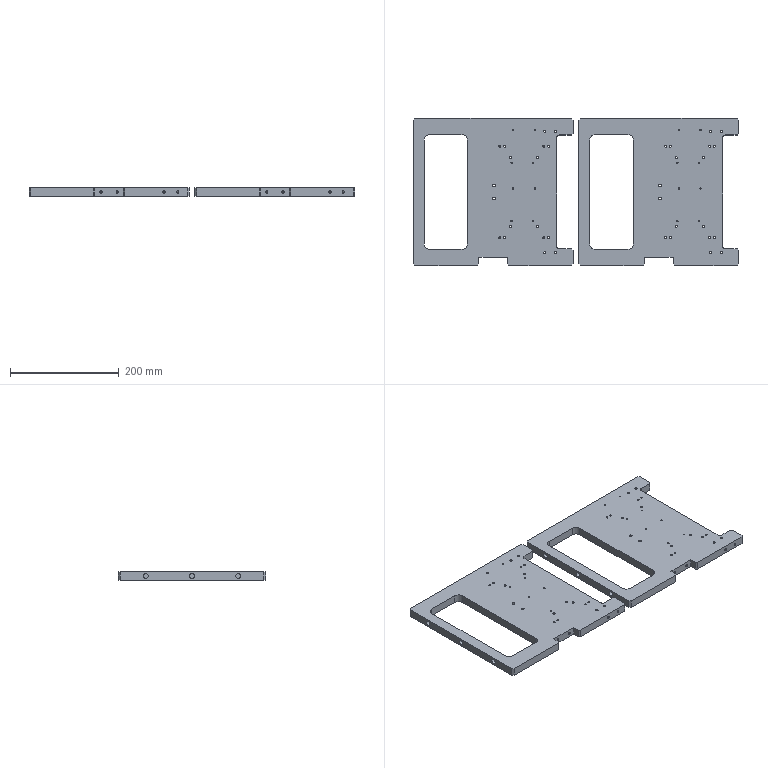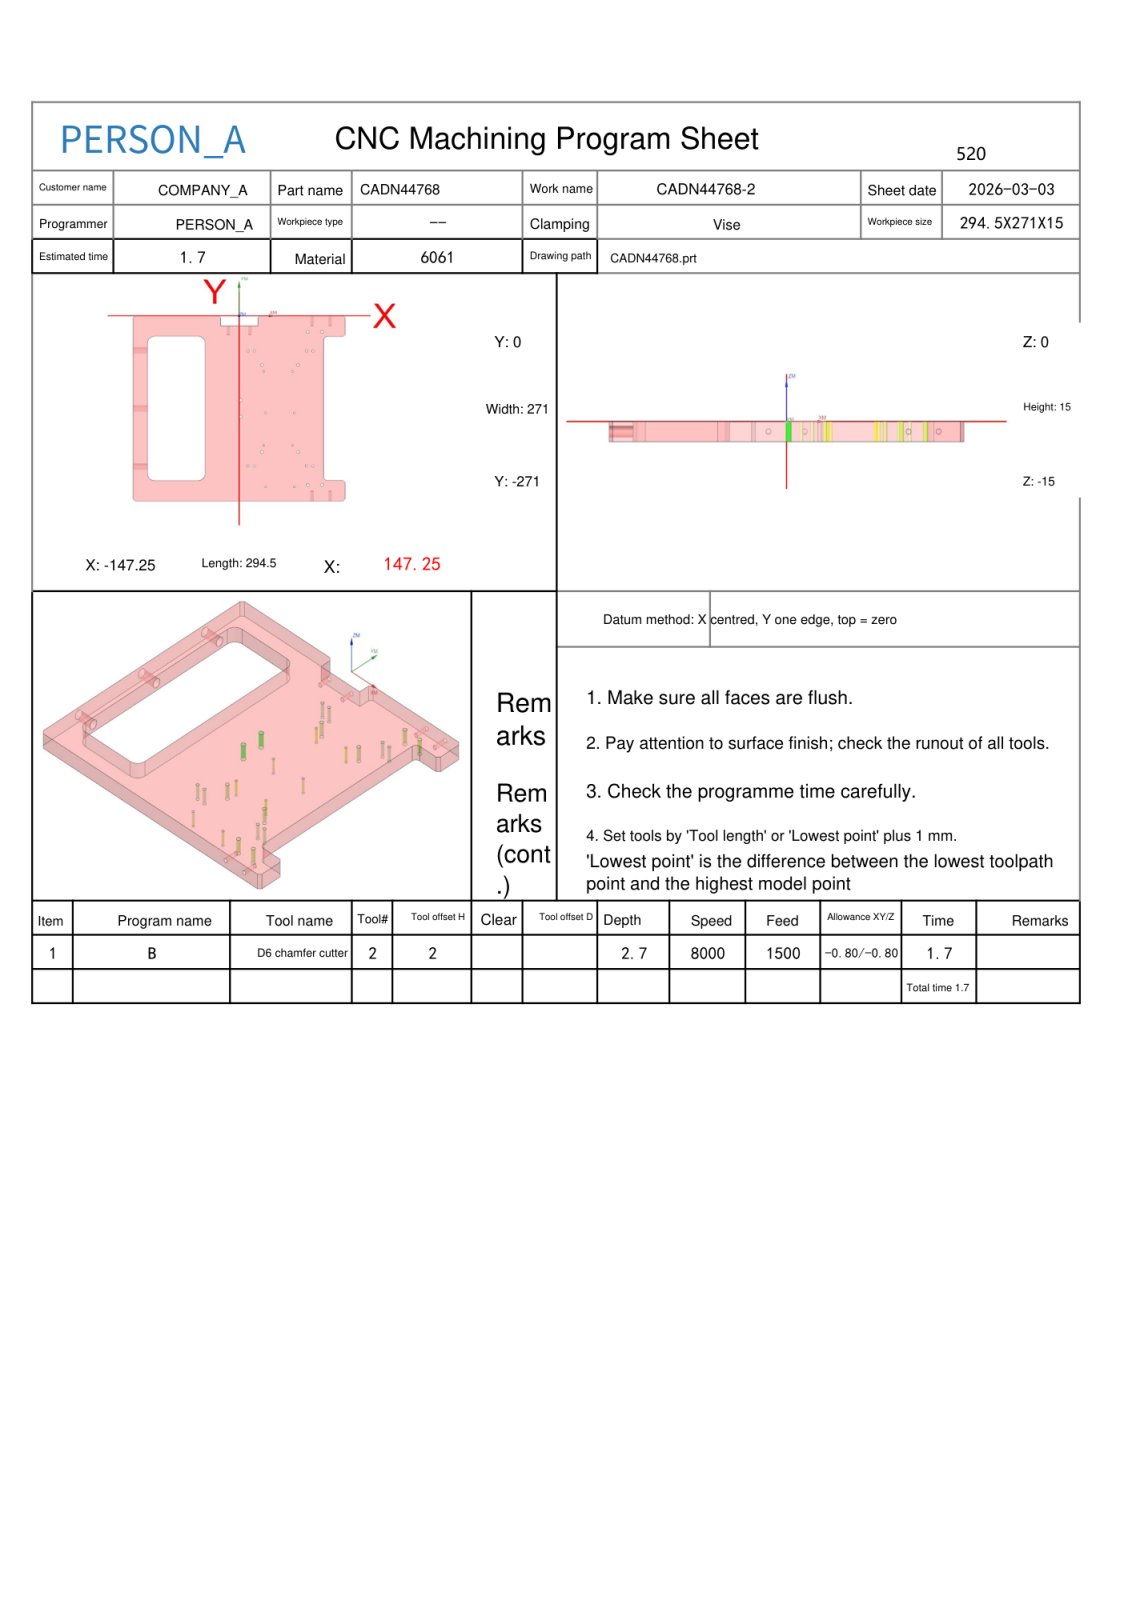NC program | NX | posted by the shop | part box 600 x 271 x 15 mm
Whole program:
%
O0001
(Machine time: 1.84 MIN)
(===Total Tool:1===)
(T2=D6 chamfer cutter   D=6.   R=0.   D-  H02 Z=-2.7  )
G80 G90 G17 G49 G40
G91 G28 Z0
M01
N1 T02 M06
(D6 chamfer cutter  D=6. R=0. H=02 ce=-0.30 di=0.00)
G00 G90 G54 X-122.006 Y-32.011 M03 S7000
G43 H02 Z50.
M08
Z2.5
G01 X-122.334 Y-32.209 Z2.361 F1500.
X-122.859 Y-32.578 Z2.127
X-123.358 Y-32.983 Z1.893
X-123.828 Y-33.422 Z1.659
X-124.267 Y-33.892 Z1.425
X-124.672 Y-34.391 Z1.191
X-125.041 Y-34.916 Z.957
X-125.374 Y-35.466 Z.723
X-125.667 Y-36.038 Z.489
X-125.921 Y-36.629 Z.255
X-126.133 Y-37.235 Z.022
X-126.302 Y-37.855 Z-.212
X-126.429 Y-38.485 Z-.446
X-126.512 Y-39.122 Z-.68
X-126.55 Y-39.764 Z-.914
Y-40. Z-1.
Y-231.
G03 X-117.25 Y-240.3 I9.3 J0.0
G01 X-57.25
G03 X-47.95 Y-231. I0.0 J9.3
G01 Y-40.
G03 X-57.25 Y-30.7 I-9.3 J0.0
G01 X-117.25
G03 X-126.55 Y-40. I0.0 J-9.3
G01 Y-40.5
Z1.5
G00 Z50.
G00 G90 X-147.95 Y-11.954 M03 S7000
Z50.
Z2.5
G01 Y-3.124 Z-.714 F1500.
Y-3.047 Z-.742
X-147.912 Y-2.84 Z-.819
X-147.831 Y-2.645 Z-.895
X-147.712 Y-2.472 Z-.972
X-147.657 Y-2.417 Z-1.
X-144.833 Y.407
G02 X-144.126 Y.7 I.707 J-.707
G01 X-29.124
G02 X-28.417 Y.407 I0.0 J-1.
G01 X-25.593 Y-2.417
G02 X-25.3 Y-3.124 I-.707 J-.707
G01 Y-14.3
X25.3
Y-3.124
G02 X25.593 Y-2.417 I1. J0.0
G01 X28.417 Y.407
G02 X29.124 Y.7 I.707 J-.707
G01 X144.126
G02 X144.833 Y.407 I0.0 J-1.
G01 X147.657 Y-2.417
G02 X147.95 Y-3.124 I-.707 J-.707
G01 Y-27.376
G02 X147.657 Y-28.083 I-1. J0.0
G01 X144.833 Y-30.907
G02 X144.126 Y-31.2 I-.707 J.707
G01 X122.25
G03 X117.95 Y-35.5 I0.0 J-4.3
G01 Y-235.5
G03 X122.25 Y-239.8 I4.3 J0.0
G01 X144.126
G02 X144.833 Y-240.093 I0.0 J-1.
G01 X147.657 Y-242.917
G02 X147.95 Y-243.624 I-.707 J-.707
G01 Y-267.876
G02 X147.657 Y-268.583 I-1. J0.0
G01 X144.833 Y-271.407
G02 X144.126 Y-271.7 I-.707 J.707
G01 X-144.126
G02 X-144.833 Y-271.407 I0.0 J1.
G01 X-147.657 Y-268.583
G02 X-147.95 Y-267.876 I.707 J.707
G01 Y-3.124
G02 X-147.657 Y-2.417 I1. J0.0
G01 X-147.304 Y-2.064
Z1.5
G00 Z50.
G00 G90 X36.75 Y-250. M03 S8000
Z50.
G98 G81 X36.75 Y-250. Z-1.75 R3. F1000.
X76.75
X74. Y-189.5
X34.
X36.75 Y-142.
X76.75
X74. Y-81.5
X34.
G80
G00 Z50.
G00 G90 X102.25 Y-219.5 M03 S8000
Z50.
G98 G81 X102.25 Y-219.5 Z-2.2 R3. F1000.
X93.25
X21.25
X12.25
Y-51.5
X21.25
X93.25
X102.25
G80
G00 Z50.
G00 G90 X31.75 Y-72. M03 S8000
Z50.
G98 G81 X31.75 Y-72. Z-2.3 R3. F1000.
X81.75
Y-199.
X31.75
G80
G00 Z50.
G00 G90 X115.25 Y-23.5 M03 S8000
Z50.
G98 G81 X115.25 Y-23.5 Z-2.7 R3. F1000.
X95.25
Y-247.5
X115.25
G80
G00 Z50.
G00 G90 X.695 Y-124.959 M03 S7000
Z50.
Z2.5
G01 X.732 Y-124.988 Z2.483 F1500.
X.97 Y-125.125 Z2.383
X1.225 Y-125.225 Z2.283
X1.493 Y-125.285 Z2.183
X1.767 Y-125.303 Z2.084
X2.04 Y-125.28 Z1.984
X2.306 Y-125.215 Z1.884
X2.56 Y-125.111 Z1.784
X2.74 Y-125.007 Z1.708
X2.957 Y-124.839 Z1.609
X3.146 Y-124.641 Z1.509
X3.303 Y-124.416 Z1.409
X3.424 Y-124.17 Z1.309
X3.506 Y-123.908 Z1.209
X3.548 Y-123.637 Z1.11
Y-123.363 Z1.01
X3.506 Y-123.092 Z.91
X3.424 Y-122.83 Z.81
X3.303 Y-122.584 Z.71
X3.146 Y-122.359 Z.611
X2.957 Y-122.161 Z.511
X2.74 Y-121.993 Z.411
X2.56 Y-121.889 Z.335
X2.306 Y-121.785 Z.235
X2.04 Y-121.72 Z.136
X1.767 Y-121.697 Z.036
X1.493 Y-121.715 Z-.064
X1.225 Y-121.775 Z-.164
X.97 Y-121.875 Z-.264
X.732 Y-122.012 Z-.363
X.518 Y-122.183 Z-.463
X.333 Y-122.385 Z-.563
X.18 Y-122.613 Z-.663
X.064 Y-122.861 Z-.763
X-.013 Y-123.124 Z-.862
X-.05 Y-123.396 Z-.962
Y-123.5 Z-1.
G03 X1.75 Y-125.3 I1.8 J0.0
X3.55 Y-123.5 I0.0 J1.8
X1.75 Y-121.7 I-1.8 J0.0
X-.05 Y-123.5 I0.0 J-1.8
X.019 Y-123.994 I1.8 J0.0
G01 Z1.5
G00 Z50.
X.695 Y-148.959
Z2.5
G01 X.732 Y-148.988 Z2.483
X.97 Y-149.125 Z2.383
X1.225 Y-149.225 Z2.283
X1.493 Y-149.285 Z2.183
X1.767 Y-149.303 Z2.084
X2.04 Y-149.28 Z1.984
X2.306 Y-149.215 Z1.884
X2.56 Y-149.111 Z1.784
X2.74 Y-149.007 Z1.708
X2.957 Y-148.839 Z1.609
X3.146 Y-148.641 Z1.509
X3.303 Y-148.416 Z1.409
X3.424 Y-148.17 Z1.309
X3.506 Y-147.908 Z1.209
X3.548 Y-147.637 Z1.11
Y-147.363 Z1.01
X3.506 Y-147.092 Z.91
X3.424 Y-146.83 Z.81
X3.303 Y-146.584 Z.71
X3.146 Y-146.359 Z.611
X2.957 Y-146.161 Z.511
X2.74 Y-145.993 Z.411
X2.56 Y-145.889 Z.335
X2.306 Y-145.785 Z.235
X2.04 Y-145.72 Z.136
X1.767 Y-145.697 Z.036
X1.493 Y-145.715 Z-.064
X1.225 Y-145.775 Z-.164
X.97 Y-145.875 Z-.264
X.732 Y-146.012 Z-.363
X.518 Y-146.183 Z-.463
X.333 Y-146.385 Z-.563
X.18 Y-146.613 Z-.663
X.064 Y-146.861 Z-.763
X-.013 Y-147.124 Z-.862
X-.05 Y-147.396 Z-.962
Y-147.5 Z-1.
G03 X1.75 Y-149.3 I1.8 J0.0
X3.55 Y-147.5 I0.0 J1.8
X1.75 Y-145.7 I-1.8 J0.0
X-.05 Y-147.5 I0.0 J-1.8
X.019 Y-147.994 I1.8 J0.0
G01 Z1.5
G00 Z50.
G00 G90 X1.982 Y-124.37 M03 S8000
Z50.
Z-.9
G01 Z-1.4 F600.
X2.15 Y-125.
G03 X3.65 Y-123.5 I0.0 J1.5
X1.75 Y-121.6 I-1.9 J0.0
X-.15 Y-123.5 I0.0 J-1.9
X1.75 Y-125.4 I1.9 J0.0
X3.65 Y-123.5 I0.0 J1.9
X2.15 Y-122. I-1.5 J0.0
G01 X1.982 Y-122.63
Z-.9
G00 Z50.
Y-148.37
Z-.9
G01 Z-1.4
X2.15 Y-149.
G03 X3.65 Y-147.5 I0.0 J1.5
X1.75 Y-145.6 I-1.9 J0.0
X-.15 Y-147.5 I0.0 J-1.9
X1.75 Y-149.4 I1.9 J0.0
X3.65 Y-147.5 I0.0 J1.9
X2.15 Y-146. I-1.5 J0.0
G01 X1.982 Y-146.63
Z-.9
G00 Z50.
M05
M09
G91 G28 Z0.0
G91 G28 Y0.0
M30
%